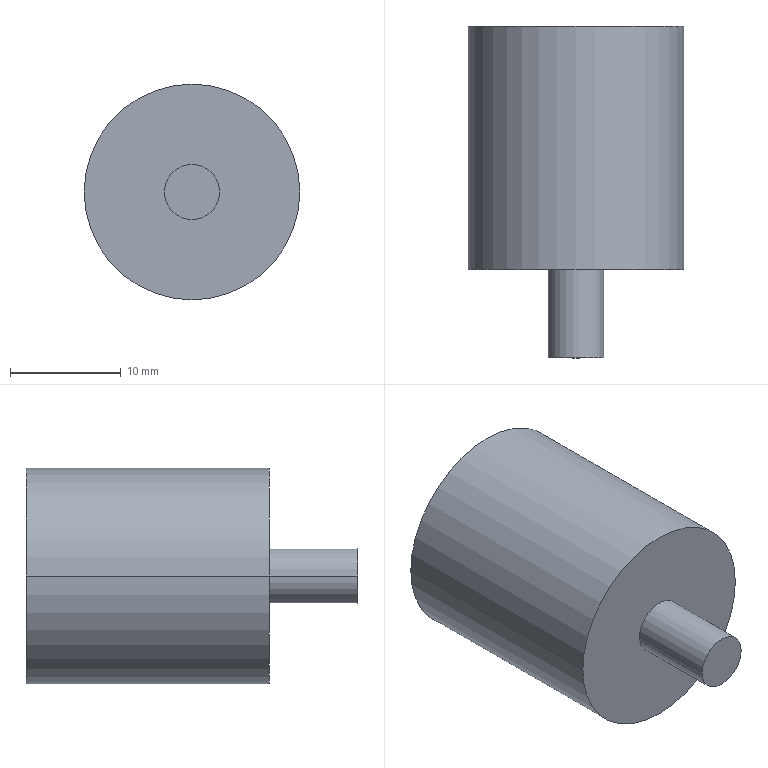Part | STEP file | LIB_57422564 | 1 solid | 10 faces | box 19.5 x 30 x 19.5 mm | volume 6600 mm3 | cylinder 6 | plane 4 | commonest cylinder face diameters 5 x4 19.5 x2
STEP:
#1=CARTESIAN_POINT('',(0.,0.,0.));
#2=DIRECTION('',(0.,0.,1.));
#3=DIRECTION('',(1.,0.,0.));
#4=AXIS2_PLACEMENT_3D('',#1,#2,#3);
#5=CARTESIAN_POINT('',(2.5,-8.,0.));
#6=VERTEX_POINT('',#5);
#7=CARTESIAN_POINT('',(-2.5,-8.,0.));
#8=VERTEX_POINT('',#7);
#9=CARTESIAN_POINT('',(0.,-8.,0.));
#10=DIRECTION('',(0.,1.,0.));
#11=DIRECTION('',(1.,0.,0.));
#12=AXIS2_PLACEMENT_3D('',#9,#10,#11);
#13=CIRCLE('',#12,2.5);
#14=CARTESIAN_POINT('',(0.,-8.,0.));
#15=DIRECTION('',(0.,-1.,0.));
#16=DIRECTION('',(-1.,0.,0.));
#17=AXIS2_PLACEMENT_3D('',#14,#15,#16);
#18=PLANE('',#17);
#19=CARTESIAN_POINT('',(-2.5,0.));
#20=CARTESIAN_POINT('',(-2.5,4.33));
#21=CARTESIAN_POINT('',(1.25,2.165));
#22=CARTESIAN_POINT('',(5.,0.));
#23=CARTESIAN_POINT('',(1.25,-2.165));
#24=CARTESIAN_POINT('',(-2.5,-4.33));
#25=CARTESIAN_POINT('',(-2.5,0.));
#26=(BOUNDED_CURVE()B_SPLINE_CURVE(2,(#19,#20,#21,#22,#23,#24,#25),.UNSPECIFIED.,.T.,.F.)B_SPLINE_CURVE_WITH_KNOTS((1,2,2,2,2,1),(-2.094,0.,2.094,4.189,6.283,8.378),.UNSPECIFIED.)CURVE()GEOMETRIC_REPRESENTATION_ITEM()RATIONAL_B_SPLINE_CURVE((1.,0.5,1.,0.5,1.,0.5,1.))REPRESENTATION_ITEM(''));
#27=(GEOMETRIC_REPRESENTATION_CONTEXT(2)PARAMETRIC_REPRESENTATION_CONTEXT()REPRESENTATION_CONTEXT('',''));
#28=DEFINITIONAL_REPRESENTATION('',(#26),#27);
#29=PCURVE('',#18,#28);
#30=CARTESIAN_POINT('',(0.,23.5,0.));
#31=DIRECTION('',(0.,-1.,0.));
#32=DIRECTION('',(-1.,0.,0.));
#33=AXIS2_PLACEMENT_3D('',#30,#31,#32);
#34=CYLINDRICAL_SURFACE('',#33,2.5);
#35=CARTESIAN_POINT('',(3.142,31.5));
#36=DIRECTION('',(-1.,0.));
#37=VECTOR('',#36,1.);
#38=LINE('',#35,#37);
#39=(GEOMETRIC_REPRESENTATION_CONTEXT(2)PARAMETRIC_REPRESENTATION_CONTEXT()REPRESENTATION_CONTEXT('',''));
#40=DEFINITIONAL_REPRESENTATION('',(#38),#39);
#41=PCURVE('',#34,#40);
#42=SURFACE_CURVE('',#13,(#29,#41),.PCURVE_S1.);
#43=EDGE_CURVE('',#6,#8,#42,.T.);
#44=ORIENTED_EDGE('',*,*,#43,.T.);
#45=CARTESIAN_POINT('',(0.,-8.,0.));
#46=DIRECTION('',(0.,-1.,0.));
#47=DIRECTION('',(1.,0.,0.));
#48=AXIS2_PLACEMENT_3D('',#45,#46,#47);
#49=CIRCLE('',#48,2.5);
#50=CARTESIAN_POINT('',(0.,0.));
#51=DIRECTION('',(-1.,0.));
#52=AXIS2_PLACEMENT_2D('',#50,#51);
#53=CIRCLE('',#52,2.5);
#54=(GEOMETRIC_REPRESENTATION_CONTEXT(2)PARAMETRIC_REPRESENTATION_CONTEXT()REPRESENTATION_CONTEXT('',''));
#55=DEFINITIONAL_REPRESENTATION('',(#53),#54);
#56=PCURVE('',#18,#55);
#57=CARTESIAN_POINT('',(0.,23.5,0.));
#58=DIRECTION('',(0.,-1.,0.));
#59=DIRECTION('',(-1.,0.,0.));
#60=AXIS2_PLACEMENT_3D('',#57,#58,#59);
#61=CYLINDRICAL_SURFACE('',#60,2.5);
#62=CARTESIAN_POINT('',(3.142,31.5));
#63=DIRECTION('',(1.,0.));
#64=VECTOR('',#63,1.);
#65=LINE('',#62,#64);
#66=(GEOMETRIC_REPRESENTATION_CONTEXT(2)PARAMETRIC_REPRESENTATION_CONTEXT()REPRESENTATION_CONTEXT('',''));
#67=DEFINITIONAL_REPRESENTATION('',(#65),#66);
#68=PCURVE('',#61,#67);
#69=SURFACE_CURVE('',#49,(#56,#68),.PCURVE_S1.);
#70=EDGE_CURVE('',#6,#8,#69,.T.);
#71=ORIENTED_EDGE('',*,*,#70,.F.);
#72=EDGE_LOOP('',(#44,#71));
#73=FACE_BOUND('',#72,.F.);
#74=ADVANCED_FACE('',(#73),#18,.T.);
#75=ORIENTED_EDGE('',*,*,#43,.T.);
#76=CARTESIAN_POINT('',(-2.5,0.,0.));
#77=VERTEX_POINT('',#76);
#78=CARTESIAN_POINT('',(-2.5,-8.,0.));
#79=DIRECTION('',(0.,1.,0.));
#80=VECTOR('',#79,1.);
#81=LINE('',#78,#80);
#82=CARTESIAN_POINT('',(0.,31.5));
#83=DIRECTION('',(0.,-1.));
#84=VECTOR('',#83,1.);
#85=LINE('',#82,#84);
#86=(GEOMETRIC_REPRESENTATION_CONTEXT(2)PARAMETRIC_REPRESENTATION_CONTEXT()REPRESENTATION_CONTEXT('',''));
#87=DEFINITIONAL_REPRESENTATION('',(#85),#86);
#88=PCURVE('',#34,#87);
#89=CARTESIAN_POINT('',(6.283,31.5));
#90=DIRECTION('',(0.,-1.));
#91=VECTOR('',#90,1.);
#92=LINE('',#89,#91);
#93=(GEOMETRIC_REPRESENTATION_CONTEXT(2)PARAMETRIC_REPRESENTATION_CONTEXT()REPRESENTATION_CONTEXT('',''));
#94=DEFINITIONAL_REPRESENTATION('',(#92),#93);
#95=PCURVE('',#61,#94);
#96=SURFACE_CURVE('',#81,(#88,#95),.PCURVE_S1.);
#97=EDGE_CURVE('',#8,#77,#96,.T.);
#98=ORIENTED_EDGE('',*,*,#97,.T.);
#99=CARTESIAN_POINT('',(2.5,0.,0.));
#100=VERTEX_POINT('',#99);
#101=CARTESIAN_POINT('',(0.,0.,0.));
#102=DIRECTION('',(0.,1.,0.));
#103=DIRECTION('',(1.,0.,0.));
#104=AXIS2_PLACEMENT_3D('',#101,#102,#103);
#105=CIRCLE('',#104,2.5);
#106=CARTESIAN_POINT('',(3.142,23.5));
#107=DIRECTION('',(-1.,0.));
#108=VECTOR('',#107,1.);
#109=LINE('',#106,#108);
#110=(GEOMETRIC_REPRESENTATION_CONTEXT(2)PARAMETRIC_REPRESENTATION_CONTEXT()REPRESENTATION_CONTEXT('',''));
#111=DEFINITIONAL_REPRESENTATION('',(#109),#110);
#112=PCURVE('',#34,#111);
#113=CARTESIAN_POINT('',(0.,0.,0.));
#114=DIRECTION('',(0.,-1.,0.));
#115=DIRECTION('',(-1.,0.,0.));
#116=AXIS2_PLACEMENT_3D('',#113,#114,#115);
#117=PLANE('',#116);
#118=CARTESIAN_POINT('',(-2.5,0.));
#119=CARTESIAN_POINT('',(-2.5,4.33));
#120=CARTESIAN_POINT('',(1.25,2.165));
#121=CARTESIAN_POINT('',(5.,0.));
#122=CARTESIAN_POINT('',(1.25,-2.165));
#123=CARTESIAN_POINT('',(-2.5,-4.33));
#124=CARTESIAN_POINT('',(-2.5,0.));
#125=(BOUNDED_CURVE()B_SPLINE_CURVE(2,(#118,#119,#120,#121,#122,#123,#124),.UNSPECIFIED.,.T.,.F.)B_SPLINE_CURVE_WITH_KNOTS((1,2,2,2,2,1),(-2.094,0.,2.094,4.189,6.283,8.378),.UNSPECIFIED.)CURVE()GEOMETRIC_REPRESENTATION_ITEM()RATIONAL_B_SPLINE_CURVE((1.,0.5,1.,0.5,1.,0.5,1.))REPRESENTATION_ITEM(''));
#126=(GEOMETRIC_REPRESENTATION_CONTEXT(2)PARAMETRIC_REPRESENTATION_CONTEXT()REPRESENTATION_CONTEXT('',''));
#127=DEFINITIONAL_REPRESENTATION('',(#125),#126);
#128=PCURVE('',#117,#127);
#129=SURFACE_CURVE('',#105,(#112,#128),.PCURVE_S1.);
#130=EDGE_CURVE('',#100,#77,#129,.T.);
#131=ORIENTED_EDGE('',*,*,#130,.F.);
#132=CARTESIAN_POINT('',(2.5,-8.,0.));
#133=DIRECTION('',(0.,1.,0.));
#134=VECTOR('',#133,1.);
#135=LINE('',#132,#134);
#136=CARTESIAN_POINT('',(3.142,31.5));
#137=DIRECTION('',(0.,-1.));
#138=VECTOR('',#137,1.);
#139=LINE('',#136,#138);
#140=(GEOMETRIC_REPRESENTATION_CONTEXT(2)PARAMETRIC_REPRESENTATION_CONTEXT()REPRESENTATION_CONTEXT('',''));
#141=DEFINITIONAL_REPRESENTATION('',(#139),#140);
#142=PCURVE('',#34,#141);
#143=CARTESIAN_POINT('',(3.142,31.5));
#144=DIRECTION('',(0.,-1.));
#145=VECTOR('',#144,1.);
#146=LINE('',#143,#145);
#147=(GEOMETRIC_REPRESENTATION_CONTEXT(2)PARAMETRIC_REPRESENTATION_CONTEXT()REPRESENTATION_CONTEXT('',''));
#148=DEFINITIONAL_REPRESENTATION('',(#146),#147);
#149=PCURVE('',#61,#148);
#150=SURFACE_CURVE('',#135,(#142,#149),.PCURVE_S1.);
#151=EDGE_CURVE('',#6,#100,#150,.T.);
#152=ORIENTED_EDGE('',*,*,#151,.F.);
#153=EDGE_LOOP('',(#75,#98,#131,#152));
#154=FACE_BOUND('',#153,.T.);
#155=ADVANCED_FACE('',(#154),#34,.T.);
#156=CARTESIAN_POINT('',(0.,0.,0.));
#157=DIRECTION('',(0.,-1.,0.));
#158=DIRECTION('',(1.,0.,0.));
#159=AXIS2_PLACEMENT_3D('',#156,#157,#158);
#160=CIRCLE('',#159,2.5);
#161=CARTESIAN_POINT('',(3.142,23.5));
#162=DIRECTION('',(1.,0.));
#163=VECTOR('',#162,1.);
#164=LINE('',#161,#163);
#165=(GEOMETRIC_REPRESENTATION_CONTEXT(2)PARAMETRIC_REPRESENTATION_CONTEXT()REPRESENTATION_CONTEXT('',''));
#166=DEFINITIONAL_REPRESENTATION('',(#164),#165);
#167=PCURVE('',#61,#166);
#168=CARTESIAN_POINT('',(0.,0.));
#169=DIRECTION('',(-1.,0.));
#170=AXIS2_PLACEMENT_2D('',#168,#169);
#171=CIRCLE('',#170,2.5);
#172=(GEOMETRIC_REPRESENTATION_CONTEXT(2)PARAMETRIC_REPRESENTATION_CONTEXT()REPRESENTATION_CONTEXT('',''));
#173=DEFINITIONAL_REPRESENTATION('',(#171),#172);
#174=PCURVE('',#117,#173);
#175=SURFACE_CURVE('',#160,(#167,#174),.PCURVE_S1.);
#176=EDGE_CURVE('',#100,#77,#175,.T.);
#177=ORIENTED_EDGE('',*,*,#176,.T.);
#178=ORIENTED_EDGE('',*,*,#97,.F.);
#179=ORIENTED_EDGE('',*,*,#70,.F.);
#180=ORIENTED_EDGE('',*,*,#151,.T.);
#181=EDGE_LOOP('',(#177,#178,#179,#180));
#182=FACE_BOUND('',#181,.T.);
#183=ADVANCED_FACE('',(#182),#61,.T.);
#184=CARTESIAN_POINT('',(9.75,0.,0.));
#185=VERTEX_POINT('',#184);
#186=CARTESIAN_POINT('',(-9.75,0.,0.));
#187=VERTEX_POINT('',#186);
#188=CARTESIAN_POINT('',(0.,0.,0.));
#189=DIRECTION('',(0.,1.,0.));
#190=DIRECTION('',(1.,0.,0.));
#191=AXIS2_PLACEMENT_3D('',#188,#189,#190);
#192=CIRCLE('',#191,9.75);
#193=CARTESIAN_POINT('',(-9.75,0.));
#194=CARTESIAN_POINT('',(-9.75,16.887));
#195=CARTESIAN_POINT('',(4.875,8.444));
#196=CARTESIAN_POINT('',(19.5,0.));
#197=CARTESIAN_POINT('',(4.875,-8.444));
#198=CARTESIAN_POINT('',(-9.75,-16.887));
#199=CARTESIAN_POINT('',(-9.75,0.));
#200=(BOUNDED_CURVE()B_SPLINE_CURVE(2,(#193,#194,#195,#196,#197,#198,#199),.UNSPECIFIED.,.T.,.F.)B_SPLINE_CURVE_WITH_KNOTS((1,2,2,2,2,1),(-2.094,0.,2.094,4.189,6.283,8.378),.UNSPECIFIED.)CURVE()GEOMETRIC_REPRESENTATION_ITEM()RATIONAL_B_SPLINE_CURVE((1.,0.5,1.,0.5,1.,0.5,1.))REPRESENTATION_ITEM(''));
#201=(GEOMETRIC_REPRESENTATION_CONTEXT(2)PARAMETRIC_REPRESENTATION_CONTEXT()REPRESENTATION_CONTEXT('',''));
#202=DEFINITIONAL_REPRESENTATION('',(#200),#201);
#203=PCURVE('',#117,#202);
#204=CARTESIAN_POINT('',(0.,23.5,0.));
#205=DIRECTION('',(0.,-1.,0.));
#206=DIRECTION('',(-1.,0.,0.));
#207=AXIS2_PLACEMENT_3D('',#204,#205,#206);
#208=CYLINDRICAL_SURFACE('',#207,9.75);
#209=CARTESIAN_POINT('',(3.142,23.5));
#210=DIRECTION('',(-1.,0.));
#211=VECTOR('',#210,1.);
#212=LINE('',#209,#211);
#213=(GEOMETRIC_REPRESENTATION_CONTEXT(2)PARAMETRIC_REPRESENTATION_CONTEXT()REPRESENTATION_CONTEXT('',''));
#214=DEFINITIONAL_REPRESENTATION('',(#212),#213);
#215=PCURVE('',#208,#214);
#216=SURFACE_CURVE('',#192,(#203,#215),.PCURVE_S1.);
#217=EDGE_CURVE('',#185,#187,#216,.T.);
#218=ORIENTED_EDGE('',*,*,#217,.T.);
#219=CARTESIAN_POINT('',(0.,0.,0.));
#220=DIRECTION('',(0.,-1.,0.));
#221=DIRECTION('',(1.,0.,0.));
#222=AXIS2_PLACEMENT_3D('',#219,#220,#221);
#223=CIRCLE('',#222,9.75);
#224=CARTESIAN_POINT('',(0.,0.));
#225=DIRECTION('',(-1.,0.));
#226=AXIS2_PLACEMENT_2D('',#224,#225);
#227=CIRCLE('',#226,9.75);
#228=(GEOMETRIC_REPRESENTATION_CONTEXT(2)PARAMETRIC_REPRESENTATION_CONTEXT()REPRESENTATION_CONTEXT('',''));
#229=DEFINITIONAL_REPRESENTATION('',(#227),#228);
#230=PCURVE('',#117,#229);
#231=CARTESIAN_POINT('',(0.,23.5,0.));
#232=DIRECTION('',(0.,-1.,0.));
#233=DIRECTION('',(-1.,0.,0.));
#234=AXIS2_PLACEMENT_3D('',#231,#232,#233);
#235=CYLINDRICAL_SURFACE('',#234,9.75);
#236=CARTESIAN_POINT('',(3.142,23.5));
#237=DIRECTION('',(1.,0.));
#238=VECTOR('',#237,1.);
#239=LINE('',#236,#238);
#240=(GEOMETRIC_REPRESENTATION_CONTEXT(2)PARAMETRIC_REPRESENTATION_CONTEXT()REPRESENTATION_CONTEXT('',''));
#241=DEFINITIONAL_REPRESENTATION('',(#239),#240);
#242=PCURVE('',#235,#241);
#243=SURFACE_CURVE('',#223,(#230,#242),.PCURVE_S1.);
#244=EDGE_CURVE('',#185,#187,#243,.T.);
#245=ORIENTED_EDGE('',*,*,#244,.F.);
#246=EDGE_LOOP('',(#218,#245));
#247=FACE_BOUND('',#246,.F.);
#248=ORIENTED_EDGE('',*,*,#176,.T.);
#249=ORIENTED_EDGE('',*,*,#130,.F.);
#250=EDGE_LOOP('',(#248,#249));
#251=FACE_BOUND('',#250,.F.);
#252=ADVANCED_FACE('',(#247,#251),#117,.T.);
#253=ORIENTED_EDGE('',*,*,#217,.T.);
#254=CARTESIAN_POINT('',(-9.75,22.,0.));
#255=VERTEX_POINT('',#254);
#256=CARTESIAN_POINT('',(-9.75,0.,0.));
#257=DIRECTION('',(0.,1.,0.));
#258=VECTOR('',#257,1.);
#259=LINE('',#256,#258);
#260=CARTESIAN_POINT('',(0.,23.5));
#261=DIRECTION('',(0.,-1.));
#262=VECTOR('',#261,1.);
#263=LINE('',#260,#262);
#264=(GEOMETRIC_REPRESENTATION_CONTEXT(2)PARAMETRIC_REPRESENTATION_CONTEXT()REPRESENTATION_CONTEXT('',''));
#265=DEFINITIONAL_REPRESENTATION('',(#263),#264);
#266=PCURVE('',#208,#265);
#267=CARTESIAN_POINT('',(6.283,23.5));
#268=DIRECTION('',(0.,-1.));
#269=VECTOR('',#268,1.);
#270=LINE('',#267,#269);
#271=(GEOMETRIC_REPRESENTATION_CONTEXT(2)PARAMETRIC_REPRESENTATION_CONTEXT()REPRESENTATION_CONTEXT('',''));
#272=DEFINITIONAL_REPRESENTATION('',(#270),#271);
#273=PCURVE('',#235,#272);
#274=SURFACE_CURVE('',#259,(#266,#273),.PCURVE_S1.);
#275=EDGE_CURVE('',#187,#255,#274,.T.);
#276=ORIENTED_EDGE('',*,*,#275,.T.);
#277=CARTESIAN_POINT('',(9.75,22.,0.));
#278=VERTEX_POINT('',#277);
#279=CARTESIAN_POINT('',(0.,22.,0.));
#280=DIRECTION('',(0.,1.,0.));
#281=DIRECTION('',(1.,0.,0.));
#282=AXIS2_PLACEMENT_3D('',#279,#280,#281);
#283=CIRCLE('',#282,9.75);
#284=CARTESIAN_POINT('',(3.142,1.5));
#285=DIRECTION('',(-1.,0.));
#286=VECTOR('',#285,1.);
#287=LINE('',#284,#286);
#288=(GEOMETRIC_REPRESENTATION_CONTEXT(2)PARAMETRIC_REPRESENTATION_CONTEXT()REPRESENTATION_CONTEXT('',''));
#289=DEFINITIONAL_REPRESENTATION('',(#287),#288);
#290=PCURVE('',#208,#289);
#291=CARTESIAN_POINT('',(0.,22.,0.));
#292=DIRECTION('',(0.,-1.,0.));
#293=DIRECTION('',(-1.,0.,0.));
#294=AXIS2_PLACEMENT_3D('',#291,#292,#293);
#295=PLANE('',#294);
#296=CARTESIAN_POINT('',(-9.75,0.));
#297=CARTESIAN_POINT('',(-9.75,16.887));
#298=CARTESIAN_POINT('',(4.875,8.444));
#299=CARTESIAN_POINT('',(19.5,0.));
#300=CARTESIAN_POINT('',(4.875,-8.444));
#301=CARTESIAN_POINT('',(-9.75,-16.887));
#302=CARTESIAN_POINT('',(-9.75,0.));
#303=(BOUNDED_CURVE()B_SPLINE_CURVE(2,(#296,#297,#298,#299,#300,#301,#302),.UNSPECIFIED.,.T.,.F.)B_SPLINE_CURVE_WITH_KNOTS((1,2,2,2,2,1),(-2.094,0.,2.094,4.189,6.283,8.378),.UNSPECIFIED.)CURVE()GEOMETRIC_REPRESENTATION_ITEM()RATIONAL_B_SPLINE_CURVE((1.,0.5,1.,0.5,1.,0.5,1.))REPRESENTATION_ITEM(''));
#304=(GEOMETRIC_REPRESENTATION_CONTEXT(2)PARAMETRIC_REPRESENTATION_CONTEXT()REPRESENTATION_CONTEXT('',''));
#305=DEFINITIONAL_REPRESENTATION('',(#303),#304);
#306=PCURVE('',#295,#305);
#307=SURFACE_CURVE('',#283,(#290,#306),.PCURVE_S1.);
#308=EDGE_CURVE('',#278,#255,#307,.T.);
#309=ORIENTED_EDGE('',*,*,#308,.F.);
#310=CARTESIAN_POINT('',(9.75,0.,0.));
#311=DIRECTION('',(0.,1.,0.));
#312=VECTOR('',#311,1.);
#313=LINE('',#310,#312);
#314=CARTESIAN_POINT('',(3.142,23.5));
#315=DIRECTION('',(0.,-1.));
#316=VECTOR('',#315,1.);
#317=LINE('',#314,#316);
#318=(GEOMETRIC_REPRESENTATION_CONTEXT(2)PARAMETRIC_REPRESENTATION_CONTEXT()REPRESENTATION_CONTEXT('',''));
#319=DEFINITIONAL_REPRESENTATION('',(#317),#318);
#320=PCURVE('',#208,#319);
#321=CARTESIAN_POINT('',(3.142,23.5));
#322=DIRECTION('',(0.,-1.));
#323=VECTOR('',#322,1.);
#324=LINE('',#321,#323);
#325=(GEOMETRIC_REPRESENTATION_CONTEXT(2)PARAMETRIC_REPRESENTATION_CONTEXT()REPRESENTATION_CONTEXT('',''));
#326=DEFINITIONAL_REPRESENTATION('',(#324),#325);
#327=PCURVE('',#235,#326);
#328=SURFACE_CURVE('',#313,(#320,#327),.PCURVE_S1.);
#329=EDGE_CURVE('',#185,#278,#328,.T.);
#330=ORIENTED_EDGE('',*,*,#329,.F.);
#331=EDGE_LOOP('',(#253,#276,#309,#330));
#332=FACE_BOUND('',#331,.T.);
#333=ADVANCED_FACE('',(#332),#208,.T.);
#334=CARTESIAN_POINT('',(0.,22.,0.));
#335=DIRECTION('',(0.,-1.,0.));
#336=DIRECTION('',(1.,0.,0.));
#337=AXIS2_PLACEMENT_3D('',#334,#335,#336);
#338=CIRCLE('',#337,9.75);
#339=CARTESIAN_POINT('',(3.142,1.5));
#340=DIRECTION('',(1.,0.));
#341=VECTOR('',#340,1.);
#342=LINE('',#339,#341);
#343=(GEOMETRIC_REPRESENTATION_CONTEXT(2)PARAMETRIC_REPRESENTATION_CONTEXT()REPRESENTATION_CONTEXT('',''));
#344=DEFINITIONAL_REPRESENTATION('',(#342),#343);
#345=PCURVE('',#235,#344);
#346=CARTESIAN_POINT('',(0.,0.));
#347=DIRECTION('',(-1.,0.));
#348=AXIS2_PLACEMENT_2D('',#346,#347);
#349=CIRCLE('',#348,9.75);
#350=(GEOMETRIC_REPRESENTATION_CONTEXT(2)PARAMETRIC_REPRESENTATION_CONTEXT()REPRESENTATION_CONTEXT('',''));
#351=DEFINITIONAL_REPRESENTATION('',(#349),#350);
#352=PCURVE('',#295,#351);
#353=SURFACE_CURVE('',#338,(#345,#352),.PCURVE_S1.);
#354=EDGE_CURVE('',#278,#255,#353,.T.);
#355=ORIENTED_EDGE('',*,*,#354,.T.);
#356=ORIENTED_EDGE('',*,*,#275,.F.);
#357=ORIENTED_EDGE('',*,*,#244,.F.);
#358=ORIENTED_EDGE('',*,*,#329,.T.);
#359=EDGE_LOOP('',(#355,#356,#357,#358));
#360=FACE_BOUND('',#359,.T.);
#361=ADVANCED_FACE('',(#360),#235,.T.);
#362=ORIENTED_EDGE('',*,*,#354,.T.);
#363=ORIENTED_EDGE('',*,*,#308,.F.);
#364=EDGE_LOOP('',(#362,#363));
#365=FACE_BOUND('',#364,.F.);
#366=CARTESIAN_POINT('',(2.5,22.,0.));
#367=VERTEX_POINT('',#366);
#368=CARTESIAN_POINT('',(-2.5,22.,0.));
#369=VERTEX_POINT('',#368);
#370=CARTESIAN_POINT('',(0.,22.,0.));
#371=DIRECTION('',(0.,1.,0.));
#372=DIRECTION('',(1.,0.,0.));
#373=AXIS2_PLACEMENT_3D('',#370,#371,#372);
#374=CIRCLE('',#373,2.5);
#375=CARTESIAN_POINT('',(-2.5,0.));
#376=CARTESIAN_POINT('',(-2.5,4.33));
#377=CARTESIAN_POINT('',(1.25,2.165));
#378=CARTESIAN_POINT('',(5.,0.));
#379=CARTESIAN_POINT('',(1.25,-2.165));
#380=CARTESIAN_POINT('',(-2.5,-4.33));
#381=CARTESIAN_POINT('',(-2.5,0.));
#382=(BOUNDED_CURVE()B_SPLINE_CURVE(2,(#375,#376,#377,#378,#379,#380,#381),.UNSPECIFIED.,.T.,.F.)B_SPLINE_CURVE_WITH_KNOTS((1,2,2,2,2,1),(-2.094,0.,2.094,4.189,6.283,8.378),.UNSPECIFIED.)CURVE()GEOMETRIC_REPRESENTATION_ITEM()RATIONAL_B_SPLINE_CURVE((1.,0.5,1.,0.5,1.,0.5,1.))REPRESENTATION_ITEM(''));
#383=(GEOMETRIC_REPRESENTATION_CONTEXT(2)PARAMETRIC_REPRESENTATION_CONTEXT()REPRESENTATION_CONTEXT('',''));
#384=DEFINITIONAL_REPRESENTATION('',(#382),#383);
#385=PCURVE('',#295,#384);
#386=CARTESIAN_POINT('',(0.,23.5,0.));
#387=DIRECTION('',(0.,-1.,0.));
#388=DIRECTION('',(-1.,0.,0.));
#389=AXIS2_PLACEMENT_3D('',#386,#387,#388);
#390=CYLINDRICAL_SURFACE('',#389,2.5);
#391=CARTESIAN_POINT('',(3.142,1.5));
#392=DIRECTION('',(-1.,0.));
#393=VECTOR('',#392,1.);
#394=LINE('',#391,#393);
#395=(GEOMETRIC_REPRESENTATION_CONTEXT(2)PARAMETRIC_REPRESENTATION_CONTEXT()REPRESENTATION_CONTEXT('',''));
#396=DEFINITIONAL_REPRESENTATION('',(#394),#395);
#397=PCURVE('',#390,#396);
#398=SURFACE_CURVE('',#374,(#385,#397),.PCURVE_S1.);
#399=EDGE_CURVE('',#367,#369,#398,.T.);
#400=ORIENTED_EDGE('',*,*,#399,.T.);
#401=CARTESIAN_POINT('',(0.,22.,0.));
#402=DIRECTION('',(0.,-1.,0.));
#403=DIRECTION('',(1.,0.,0.));
#404=AXIS2_PLACEMENT_3D('',#401,#402,#403);
#405=CIRCLE('',#404,2.5);
#406=CARTESIAN_POINT('',(0.,0.));
#407=DIRECTION('',(-1.,0.));
#408=AXIS2_PLACEMENT_2D('',#406,#407);
#409=CIRCLE('',#408,2.5);
#410=(GEOMETRIC_REPRESENTATION_CONTEXT(2)PARAMETRIC_REPRESENTATION_CONTEXT()REPRESENTATION_CONTEXT('',''));
#411=DEFINITIONAL_REPRESENTATION('',(#409),#410);
#412=PCURVE('',#295,#411);
#413=CARTESIAN_POINT('',(0.,23.5,0.));
#414=DIRECTION('',(0.,-1.,0.));
#415=DIRECTION('',(-1.,0.,0.));
#416=AXIS2_PLACEMENT_3D('',#413,#414,#415);
#417=CYLINDRICAL_SURFACE('',#416,2.5);
#418=CARTESIAN_POINT('',(3.142,1.5));
#419=DIRECTION('',(1.,0.));
#420=VECTOR('',#419,1.);
#421=LINE('',#418,#420);
#422=(GEOMETRIC_REPRESENTATION_CONTEXT(2)PARAMETRIC_REPRESENTATION_CONTEXT()REPRESENTATION_CONTEXT('',''));
#423=DEFINITIONAL_REPRESENTATION('',(#421),#422);
#424=PCURVE('',#417,#423);
#425=SURFACE_CURVE('',#405,(#412,#424),.PCURVE_S1.);
#426=EDGE_CURVE('',#367,#369,#425,.T.);
#427=ORIENTED_EDGE('',*,*,#426,.F.);
#428=EDGE_LOOP('',(#400,#427));
#429=FACE_BOUND('',#428,.F.);
#430=ADVANCED_FACE('',(#365,#429),#295,.F.);
#431=CARTESIAN_POINT('',(2.5,15.5,0.));
#432=VERTEX_POINT('',#431);
#433=CARTESIAN_POINT('',(2.5,22.,0.));
#434=DIRECTION('',(0.,-1.,0.));
#435=VECTOR('',#434,1.);
#436=LINE('',#433,#435);
#437=CARTESIAN_POINT('',(3.142,1.5));
#438=DIRECTION('',(0.,1.));
#439=VECTOR('',#438,1.);
#440=LINE('',#437,#439);
#441=(GEOMETRIC_REPRESENTATION_CONTEXT(2)PARAMETRIC_REPRESENTATION_CONTEXT()REPRESENTATION_CONTEXT('',''));
#442=DEFINITIONAL_REPRESENTATION('',(#440),#441);
#443=PCURVE('',#390,#442);
#444=CARTESIAN_POINT('',(3.142,1.5));
#445=DIRECTION('',(0.,1.));
#446=VECTOR('',#445,1.);
#447=LINE('',#444,#446);
#448=(GEOMETRIC_REPRESENTATION_CONTEXT(2)PARAMETRIC_REPRESENTATION_CONTEXT()REPRESENTATION_CONTEXT('',''));
#449=DEFINITIONAL_REPRESENTATION('',(#447),#448);
#450=PCURVE('',#417,#449);
#451=SURFACE_CURVE('',#436,(#443,#450),.PCURVE_S1.);
#452=EDGE_CURVE('',#367,#432,#451,.T.);
#453=ORIENTED_EDGE('',*,*,#452,.T.);
#454=CARTESIAN_POINT('',(-2.5,15.5,0.));
#455=VERTEX_POINT('',#454);
#456=CARTESIAN_POINT('',(0.,15.5,0.));
#457=DIRECTION('',(0.,1.,0.));
#458=DIRECTION('',(1.,0.,0.));
#459=AXIS2_PLACEMENT_3D('',#456,#457,#458);
#460=CIRCLE('',#459,2.5);
#461=CARTESIAN_POINT('',(3.142,8.));
#462=DIRECTION('',(-1.,0.));
#463=VECTOR('',#462,1.);
#464=LINE('',#461,#463);
#465=(GEOMETRIC_REPRESENTATION_CONTEXT(2)PARAMETRIC_REPRESENTATION_CONTEXT()REPRESENTATION_CONTEXT('',''));
#466=DEFINITIONAL_REPRESENTATION('',(#464),#465);
#467=PCURVE('',#390,#466);
#468=CARTESIAN_POINT('',(0.,15.5,0.));
#469=DIRECTION('',(0.,-1.,0.));
#470=DIRECTION('',(-1.,0.,0.));
#471=AXIS2_PLACEMENT_3D('',#468,#469,#470);
#472=PLANE('',#471);
#473=CARTESIAN_POINT('',(-2.5,0.));
#474=CARTESIAN_POINT('',(-2.5,4.33));
#475=CARTESIAN_POINT('',(1.25,2.165));
#476=CARTESIAN_POINT('',(5.,0.));
#477=CARTESIAN_POINT('',(1.25,-2.165));
#478=CARTESIAN_POINT('',(-2.5,-4.33));
#479=CARTESIAN_POINT('',(-2.5,0.));
#480=(BOUNDED_CURVE()B_SPLINE_CURVE(2,(#473,#474,#475,#476,#477,#478,#479),.UNSPECIFIED.,.T.,.F.)B_SPLINE_CURVE_WITH_KNOTS((1,2,2,2,2,1),(-2.094,0.,2.094,4.189,6.283,8.378),.UNSPECIFIED.)CURVE()GEOMETRIC_REPRESENTATION_ITEM()RATIONAL_B_SPLINE_CURVE((1.,0.5,1.,0.5,1.,0.5,1.))REPRESENTATION_ITEM(''));
#481=(GEOMETRIC_REPRESENTATION_CONTEXT(2)PARAMETRIC_REPRESENTATION_CONTEXT()REPRESENTATION_CONTEXT('',''));
#482=DEFINITIONAL_REPRESENTATION('',(#480),#481);
#483=PCURVE('',#472,#482);
#484=SURFACE_CURVE('',#460,(#467,#483),.PCURVE_S1.);
#485=EDGE_CURVE('',#432,#455,#484,.T.);
#486=ORIENTED_EDGE('',*,*,#485,.T.);
#487=CARTESIAN_POINT('',(-2.5,22.,0.));
#488=DIRECTION('',(0.,-1.,0.));
#489=VECTOR('',#488,1.);
#490=LINE('',#487,#489);
#491=CARTESIAN_POINT('',(0.,1.5));
#492=DIRECTION('',(0.,1.));
#493=VECTOR('',#492,1.);
#494=LINE('',#491,#493);
#495=(GEOMETRIC_REPRESENTATION_CONTEXT(2)PARAMETRIC_REPRESENTATION_CONTEXT()REPRESENTATION_CONTEXT('',''));
#496=DEFINITIONAL_REPRESENTATION('',(#494),#495);
#497=PCURVE('',#390,#496);
#498=CARTESIAN_POINT('',(6.283,1.5));
#499=DIRECTION('',(0.,1.));
#500=VECTOR('',#499,1.);
#501=LINE('',#498,#500);
#502=(GEOMETRIC_REPRESENTATION_CONTEXT(2)PARAMETRIC_REPRESENTATION_CONTEXT()REPRESENTATION_CONTEXT('',''));
#503=DEFINITIONAL_REPRESENTATION('',(#501),#502);
#504=PCURVE('',#417,#503);
#505=SURFACE_CURVE('',#490,(#497,#504),.PCURVE_S1.);
#506=EDGE_CURVE('',#369,#455,#505,.T.);
#507=ORIENTED_EDGE('',*,*,#506,.F.);
#508=ORIENTED_EDGE('',*,*,#399,.F.);
#509=EDGE_LOOP('',(#453,#486,#507,#508));
#510=FACE_BOUND('',#509,.F.);
#511=ADVANCED_FACE('',(#510),#390,.F.);
#512=ORIENTED_EDGE('',*,*,#452,.F.);
#513=ORIENTED_EDGE('',*,*,#426,.T.);
#514=ORIENTED_EDGE('',*,*,#506,.T.);
#515=CARTESIAN_POINT('',(0.,15.5,0.));
#516=DIRECTION('',(0.,-1.,0.));
#517=DIRECTION('',(1.,0.,0.));
#518=AXIS2_PLACEMENT_3D('',#515,#516,#517);
#519=CIRCLE('',#518,2.5);
#520=CARTESIAN_POINT('',(3.142,8.));
#521=DIRECTION('',(1.,0.));
#522=VECTOR('',#521,1.);
#523=LINE('',#520,#522);
#524=(GEOMETRIC_REPRESENTATION_CONTEXT(2)PARAMETRIC_REPRESENTATION_CONTEXT()REPRESENTATION_CONTEXT('',''));
#525=DEFINITIONAL_REPRESENTATION('',(#523),#524);
#526=PCURVE('',#417,#525);
#527=CARTESIAN_POINT('',(0.,0.));
#528=DIRECTION('',(-1.,0.));
#529=AXIS2_PLACEMENT_2D('',#527,#528);
#530=CIRCLE('',#529,2.5);
#531=(GEOMETRIC_REPRESENTATION_CONTEXT(2)PARAMETRIC_REPRESENTATION_CONTEXT()REPRESENTATION_CONTEXT('',''));
#532=DEFINITIONAL_REPRESENTATION('',(#530),#531);
#533=PCURVE('',#472,#532);
#534=SURFACE_CURVE('',#519,(#526,#533),.PCURVE_S1.);
#535=EDGE_CURVE('',#432,#455,#534,.T.);
#536=ORIENTED_EDGE('',*,*,#535,.F.);
#537=EDGE_LOOP('',(#512,#513,#514,#536));
#538=FACE_BOUND('',#537,.F.);
#539=ADVANCED_FACE('',(#538),#417,.F.);
#540=ORIENTED_EDGE('',*,*,#485,.F.);
#541=ORIENTED_EDGE('',*,*,#535,.T.);
#542=EDGE_LOOP('',(#540,#541));
#543=FACE_BOUND('',#542,.F.);
#544=ADVANCED_FACE('',(#543),#472,.F.);
#545=CLOSED_SHELL('',(#74,#155,#183,#252,#333,#361,#430,#511,#539,#544));
#546=MANIFOLD_SOLID_BREP('',#545);
#547=(LENGTH_UNIT()NAMED_UNIT(*)SI_UNIT(.MILLI.,.METRE.));
#548=UNCERTAINTY_MEASURE_WITH_UNIT(LENGTH_MEASURE(0.0000001),#547,'','');
#549=(NAMED_UNIT(*)PLANE_ANGLE_UNIT()SI_UNIT($,.RADIAN.));
#550=(NAMED_UNIT(*)SI_UNIT($,.STERADIAN.)SOLID_ANGLE_UNIT());
#551=(GEOMETRIC_REPRESENTATION_CONTEXT(3)GLOBAL_UNCERTAINTY_ASSIGNED_CONTEXT((#548))GLOBAL_UNIT_ASSIGNED_CONTEXT((#547,#549,#550))REPRESENTATION_CONTEXT('',''));
#552=ADVANCED_BREP_SHAPE_REPRESENTATION('',(#4,#546),#551);